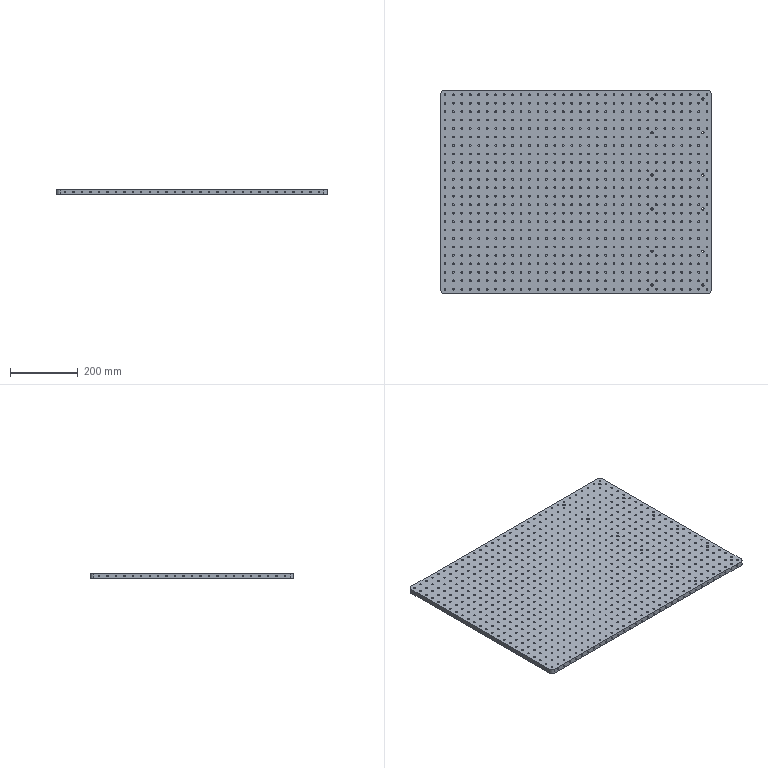Part | SolidWorks | features BaseBody 1 | 1 solid | 2698 faces | box 800 x 600 x 14 mm | volume 6524113 mm3 | cylinder 1804 | plane 894 | commonest cylinder face diameters 5.2 x1536 4.2 x216 7 x24 12 x24 20 x4